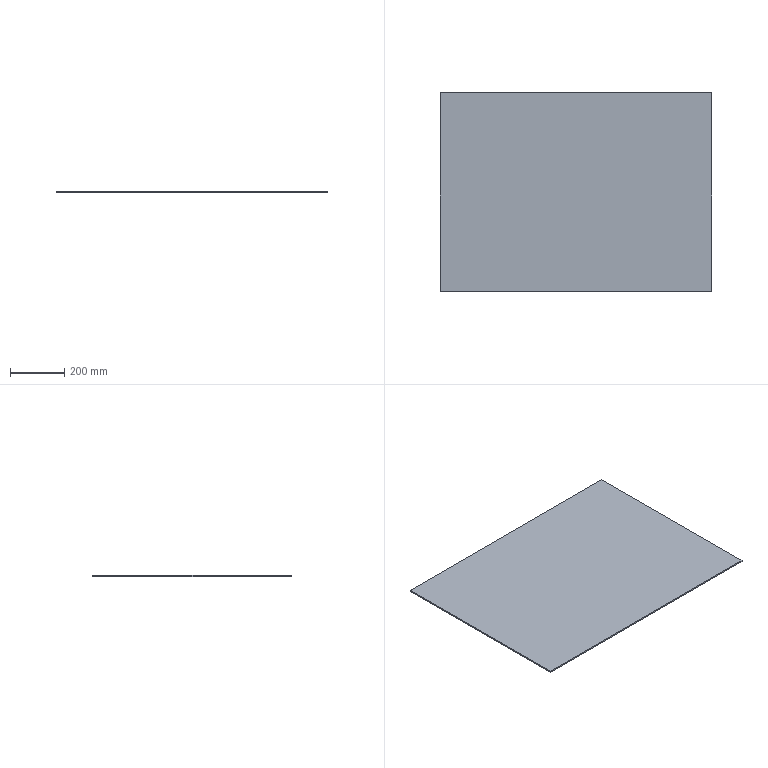Part | SolidWorks | features Extrusion 1 | 1 solid | 6 faces | box 999 x 729 x 5 mm | volume 3641355 mm3 | plane 6
STEP:
#1=CARTESIAN_POINT('',(499.5,-364.5,0.));
#2=VERTEX_POINT('',#1);
#3=CARTESIAN_POINT('',(499.5,364.5,0.));
#4=VERTEX_POINT('',#3);
#5=CARTESIAN_POINT('',(499.5,364.5,0.));
#6=DIRECTION('',(0.,1.,0.));
#7=VECTOR('',#6,1000.);
#8=LINE('',#5,#7);
#9=EDGE_CURVE('',#2,#4,#8,.T.);
#10=ORIENTED_EDGE('',*,*,#9,.T.);
#11=CARTESIAN_POINT('',(499.5,364.5,5.));
#12=VERTEX_POINT('',#11);
#13=CARTESIAN_POINT('',(499.5,364.5,5.));
#14=DIRECTION('',(0.,0.,-1.));
#15=VECTOR('',#14,1000.);
#16=LINE('',#13,#15);
#17=EDGE_CURVE('',#12,#4,#16,.T.);
#18=ORIENTED_EDGE('',*,*,#17,.F.);
#19=CARTESIAN_POINT('',(499.5,-364.5,5.));
#20=VERTEX_POINT('',#19);
#21=CARTESIAN_POINT('',(499.5,364.5,5.));
#22=DIRECTION('',(0.,1.,0.));
#23=VECTOR('',#22,1000.);
#24=LINE('',#21,#23);
#25=EDGE_CURVE('',#20,#12,#24,.T.);
#26=ORIENTED_EDGE('',*,*,#25,.F.);
#27=CARTESIAN_POINT('',(499.5,-364.5,5.));
#28=DIRECTION('',(0.,0.,-1.));
#29=VECTOR('',#28,1000.);
#30=LINE('',#27,#29);
#31=EDGE_CURVE('',#20,#2,#30,.T.);
#32=ORIENTED_EDGE('',*,*,#31,.T.);
#33=EDGE_LOOP('',(#10,#18,#26,#32));
#34=FACE_OUTER_BOUND('',#33,.T.);
#35=CARTESIAN_POINT('',(499.5,364.5,5.));
#36=DIRECTION('',(-1.,0.,0.));
#37=DIRECTION('',(0.,-1.,0.));
#38=AXIS2_PLACEMENT_3D('',#35,#36,#37);
#39=PLANE('',#38);
#40=ADVANCED_FACE('',(#34),#39,.F.);
#41=CARTESIAN_POINT('',(-499.5,364.5,0.));
#42=VERTEX_POINT('',#41);
#43=CARTESIAN_POINT('',(-499.5,364.5,0.));
#44=DIRECTION('',(-1.,0.,0.));
#45=VECTOR('',#44,1000.);
#46=LINE('',#43,#45);
#47=EDGE_CURVE('',#4,#42,#46,.T.);
#48=ORIENTED_EDGE('',*,*,#47,.T.);
#49=CARTESIAN_POINT('',(-499.5,364.5,5.));
#50=VERTEX_POINT('',#49);
#51=CARTESIAN_POINT('',(-499.5,364.5,5.));
#52=DIRECTION('',(0.,0.,-1.));
#53=VECTOR('',#52,1000.);
#54=LINE('',#51,#53);
#55=EDGE_CURVE('',#50,#42,#54,.T.);
#56=ORIENTED_EDGE('',*,*,#55,.F.);
#57=CARTESIAN_POINT('',(-499.5,364.5,5.));
#58=DIRECTION('',(-1.,0.,0.));
#59=VECTOR('',#58,1000.);
#60=LINE('',#57,#59);
#61=EDGE_CURVE('',#12,#50,#60,.T.);
#62=ORIENTED_EDGE('',*,*,#61,.F.);
#63=ORIENTED_EDGE('',*,*,#17,.T.);
#64=EDGE_LOOP('',(#48,#56,#62,#63));
#65=FACE_OUTER_BOUND('',#64,.T.);
#66=CARTESIAN_POINT('',(-499.5,364.5,5.));
#67=DIRECTION('',(0.,-1.,0.));
#68=DIRECTION('',(0.,0.,-1.));
#69=AXIS2_PLACEMENT_3D('',#66,#67,#68);
#70=PLANE('',#69);
#71=ADVANCED_FACE('',(#65),#70,.F.);
#72=CARTESIAN_POINT('',(-499.5,-364.5,0.));
#73=VERTEX_POINT('',#72);
#74=CARTESIAN_POINT('',(-499.5,364.5,0.));
#75=DIRECTION('',(0.,-1.,0.));
#76=VECTOR('',#75,1000.);
#77=LINE('',#74,#76);
#78=EDGE_CURVE('',#42,#73,#77,.T.);
#79=ORIENTED_EDGE('',*,*,#78,.T.);
#80=CARTESIAN_POINT('',(-499.5,-364.5,5.));
#81=VERTEX_POINT('',#80);
#82=CARTESIAN_POINT('',(-499.5,-364.5,5.));
#83=DIRECTION('',(0.,0.,-1.));
#84=VECTOR('',#83,1000.);
#85=LINE('',#82,#84);
#86=EDGE_CURVE('',#81,#73,#85,.T.);
#87=ORIENTED_EDGE('',*,*,#86,.F.);
#88=CARTESIAN_POINT('',(-499.5,364.5,5.));
#89=DIRECTION('',(0.,-1.,0.));
#90=VECTOR('',#89,1000.);
#91=LINE('',#88,#90);
#92=EDGE_CURVE('',#50,#81,#91,.T.);
#93=ORIENTED_EDGE('',*,*,#92,.F.);
#94=ORIENTED_EDGE('',*,*,#55,.T.);
#95=EDGE_LOOP('',(#79,#87,#93,#94));
#96=FACE_OUTER_BOUND('',#95,.T.);
#97=CARTESIAN_POINT('',(-499.5,364.5,5.));
#98=DIRECTION('',(1.,0.,0.));
#99=DIRECTION('',(0.,1.,0.));
#100=AXIS2_PLACEMENT_3D('',#97,#98,#99);
#101=PLANE('',#100);
#102=ADVANCED_FACE('',(#96),#101,.F.);
#103=CARTESIAN_POINT('',(-499.5,-364.5,0.));
#104=DIRECTION('',(1.,0.,0.));
#105=VECTOR('',#104,1000.);
#106=LINE('',#103,#105);
#107=EDGE_CURVE('',#73,#2,#106,.T.);
#108=ORIENTED_EDGE('',*,*,#107,.T.);
#109=ORIENTED_EDGE('',*,*,#31,.F.);
#110=CARTESIAN_POINT('',(-499.5,-364.5,5.));
#111=DIRECTION('',(1.,0.,0.));
#112=VECTOR('',#111,1000.);
#113=LINE('',#110,#112);
#114=EDGE_CURVE('',#81,#20,#113,.T.);
#115=ORIENTED_EDGE('',*,*,#114,.F.);
#116=ORIENTED_EDGE('',*,*,#86,.T.);
#117=EDGE_LOOP('',(#108,#109,#115,#116));
#118=FACE_OUTER_BOUND('',#117,.T.);
#119=CARTESIAN_POINT('',(-499.5,-364.5,5.));
#120=DIRECTION('',(0.,1.,0.));
#121=DIRECTION('',(0.,0.,1.));
#122=AXIS2_PLACEMENT_3D('',#119,#120,#121);
#123=PLANE('',#122);
#124=ADVANCED_FACE('',(#118),#123,.F.);
#125=ORIENTED_EDGE('',*,*,#25,.T.);
#126=ORIENTED_EDGE('',*,*,#61,.T.);
#127=ORIENTED_EDGE('',*,*,#92,.T.);
#128=ORIENTED_EDGE('',*,*,#114,.T.);
#129=EDGE_LOOP('',(#125,#126,#127,#128));
#130=FACE_OUTER_BOUND('',#129,.T.);
#131=CARTESIAN_POINT('',(0.,0.,5.));
#132=DIRECTION('',(0.,0.,1.));
#133=DIRECTION('',(1.,0.,0.));
#134=AXIS2_PLACEMENT_3D('',#131,#132,#133);
#135=PLANE('',#134);
#136=ADVANCED_FACE('',(#130),#135,.T.);
#137=ORIENTED_EDGE('',*,*,#9,.F.);
#138=ORIENTED_EDGE('',*,*,#107,.F.);
#139=ORIENTED_EDGE('',*,*,#78,.F.);
#140=ORIENTED_EDGE('',*,*,#47,.F.);
#141=EDGE_LOOP('',(#137,#138,#139,#140));
#142=FACE_OUTER_BOUND('',#141,.T.);
#143=CARTESIAN_POINT('',(0.,0.,0.));
#144=DIRECTION('',(0.,0.,1.));
#145=DIRECTION('',(1.,0.,0.));
#146=AXIS2_PLACEMENT_3D('',#143,#144,#145);
#147=PLANE('',#146);
#148=ADVANCED_FACE('',(#142),#147,.F.);
#149=CLOSED_SHELL('',(#40,#71,#102,#124,#136,#148));
#150=MANIFOLD_SOLID_BREP('',#149);
#151=CARTESIAN_POINT('',(0.,0.,0.));
#152=DIRECTION('',(0.,0.,1.));
#153=DIRECTION('',(1.,0.,0.));
#154=AXIS2_PLACEMENT_3D('',#151,#152,#153);
#155=(LENGTH_UNIT()NAMED_UNIT(*)SI_UNIT(.MILLI.,.METRE.));
#156=UNCERTAINTY_MEASURE_WITH_UNIT(LENGTH_MEASURE(0.00001),#155,'','');
#157=(NAMED_UNIT(*)PLANE_ANGLE_UNIT()SI_UNIT($,.RADIAN.));
#158=(NAMED_UNIT(*)SI_UNIT($,.STERADIAN.)SOLID_ANGLE_UNIT());
#159=(GEOMETRIC_REPRESENTATION_CONTEXT(3)GLOBAL_UNCERTAINTY_ASSIGNED_CONTEXT((#156))GLOBAL_UNIT_ASSIGNED_CONTEXT((#155,#157,#158))REPRESENTATION_CONTEXT('',''));
#160=ADVANCED_BREP_SHAPE_REPRESENTATION('',(#150,#154),#159);